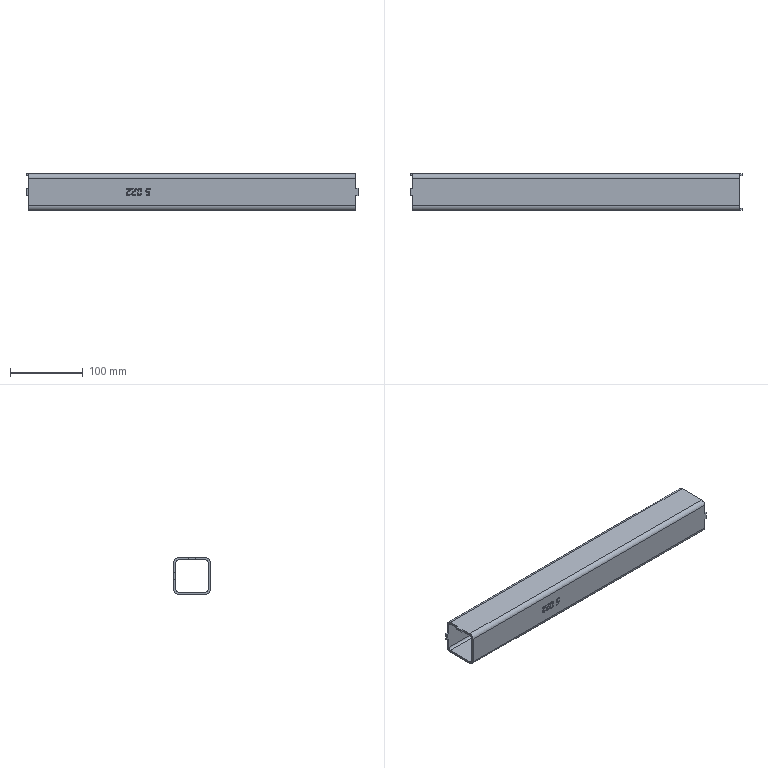Part | SolidWorks | features BaseBody 1 | 1 solid | 85 faces | box 456 x 50 x 50 mm | volume 243710 mm3 | plane 46 | spline 31 | cylinder 8 | commonest cylinder face diameters 6 x4 12 x4